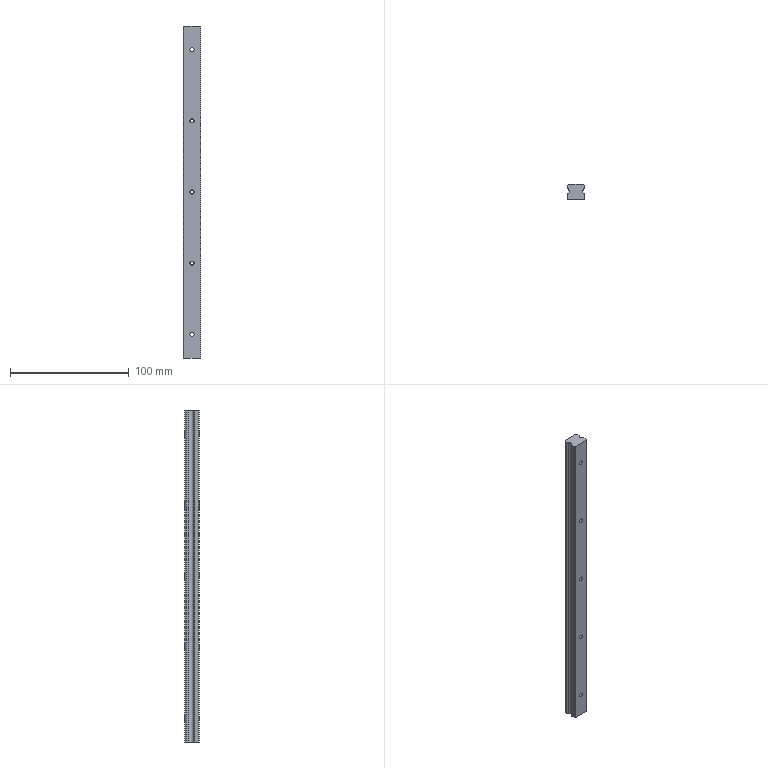Part | NX | features BREP 1 | 1 solid | 46 faces | box 15 x 12.5 x 280 mm | volume 46790 mm3 | cylinder 27 | plane 19 | commonest cylinder face diameters 3.5 x10 6 x10 3.4 x4 4 x3
STEP:
#1=CARTESIAN_POINT('',(0.,0.,-91.75));
#2=VERTEX_POINT('',#1);
#3=CARTESIAN_POINT('',(0.,0.,-88.25));
#4=VERTEX_POINT('',#3);
#5=CARTESIAN_POINT('',(0.,0.,-90.));
#6=DIRECTION('',(0.,1.,0.));
#7=DIRECTION('',(0.,0.,1.));
#8=AXIS2_PLACEMENT_3D('',#5,#6,#7);
#9=CIRCLE('',#8,1.75);
#10=EDGE_CURVE('',#2,#4,#9,.T.);
#11=ORIENTED_EDGE('',*,*,#10,.F.);
#12=CARTESIAN_POINT('',(0.,8.,-91.75));
#13=VERTEX_POINT('',#12);
#14=CARTESIAN_POINT('',(0.,0.,-91.75));
#15=DIRECTION('',(0.,1.,0.));
#16=VECTOR('',#15,1000.);
#17=LINE('',#14,#16);
#18=EDGE_CURVE('',#13,#2,#17,.F.);
#19=ORIENTED_EDGE('',*,*,#18,.F.);
#20=CARTESIAN_POINT('',(0.,8.,-88.25));
#21=VERTEX_POINT('',#20);
#22=CARTESIAN_POINT('',(0.,8.,-90.));
#23=DIRECTION('',(0.,1.,0.));
#24=DIRECTION('',(0.,0.,1.));
#25=AXIS2_PLACEMENT_3D('',#22,#23,#24);
#26=CIRCLE('',#25,1.75);
#27=EDGE_CURVE('',#13,#21,#26,.T.);
#28=ORIENTED_EDGE('',*,*,#27,.T.);
#29=CARTESIAN_POINT('',(0.,0.,-88.25));
#30=DIRECTION('',(0.,1.,0.));
#31=VECTOR('',#30,1000.);
#32=LINE('',#29,#31);
#33=EDGE_CURVE('',#21,#4,#32,.F.);
#34=ORIENTED_EDGE('',*,*,#33,.T.);
#35=EDGE_LOOP('',(#11,#19,#28,#34));
#36=FACE_BOUND('',#35,.T.);
#37=CARTESIAN_POINT('',(0.,0.,-90.));
#38=DIRECTION('',(0.,1.,0.));
#39=DIRECTION('',(0.,0.,1.));
#40=AXIS2_PLACEMENT_3D('',#37,#38,#39);
#41=CYLINDRICAL_SURFACE('',#40,1.75);
#42=ADVANCED_FACE('',(#36),#41,.F.);
#43=CARTESIAN_POINT('',(0.,8.,-93.));
#44=VERTEX_POINT('',#43);
#45=CARTESIAN_POINT('',(0.,8.,-87.));
#46=VERTEX_POINT('',#45);
#47=CARTESIAN_POINT('',(0.,8.,-90.));
#48=DIRECTION('',(0.,1.,0.));
#49=DIRECTION('',(0.,0.,1.));
#50=AXIS2_PLACEMENT_3D('',#47,#48,#49);
#51=CIRCLE('',#50,3.);
#52=EDGE_CURVE('',#44,#46,#51,.T.);
#53=ORIENTED_EDGE('',*,*,#52,.F.);
#54=CARTESIAN_POINT('',(0.,12.5,-93.));
#55=VERTEX_POINT('',#54);
#56=CARTESIAN_POINT('',(0.,0.,-93.));
#57=DIRECTION('',(0.,1.,0.));
#58=VECTOR('',#57,1000.);
#59=LINE('',#56,#58);
#60=EDGE_CURVE('',#55,#44,#59,.F.);
#61=ORIENTED_EDGE('',*,*,#60,.F.);
#62=CARTESIAN_POINT('',(0.,12.5,-87.));
#63=VERTEX_POINT('',#62);
#64=CARTESIAN_POINT('',(0.,12.5,-90.));
#65=DIRECTION('',(0.,1.,0.));
#66=DIRECTION('',(0.,0.,-1.));
#67=AXIS2_PLACEMENT_3D('',#64,#65,#66);
#68=CIRCLE('',#67,3.);
#69=EDGE_CURVE('',#55,#63,#68,.T.);
#70=ORIENTED_EDGE('',*,*,#69,.T.);
#71=CARTESIAN_POINT('',(0.,0.,-87.));
#72=DIRECTION('',(0.,1.,0.));
#73=VECTOR('',#72,1000.);
#74=LINE('',#71,#73);
#75=EDGE_CURVE('',#63,#46,#74,.F.);
#76=ORIENTED_EDGE('',*,*,#75,.T.);
#77=EDGE_LOOP('',(#53,#61,#70,#76));
#78=FACE_BOUND('',#77,.T.);
#79=CARTESIAN_POINT('',(0.,0.,-90.));
#80=DIRECTION('',(0.,1.,0.));
#81=DIRECTION('',(0.,0.,1.));
#82=AXIS2_PLACEMENT_3D('',#79,#80,#81);
#83=CYLINDRICAL_SURFACE('',#82,3.);
#84=ADVANCED_FACE('',(#78),#83,.F.);
#85=CARTESIAN_POINT('',(0.,0.,-31.75));
#86=VERTEX_POINT('',#85);
#87=CARTESIAN_POINT('',(0.,0.,-28.25));
#88=VERTEX_POINT('',#87);
#89=CARTESIAN_POINT('',(0.,0.,-30.));
#90=DIRECTION('',(0.,1.,0.));
#91=DIRECTION('',(0.,0.,1.));
#92=AXIS2_PLACEMENT_3D('',#89,#90,#91);
#93=CIRCLE('',#92,1.75);
#94=EDGE_CURVE('',#86,#88,#93,.T.);
#95=ORIENTED_EDGE('',*,*,#94,.F.);
#96=CARTESIAN_POINT('',(0.,8.,-31.75));
#97=VERTEX_POINT('',#96);
#98=CARTESIAN_POINT('',(0.,0.,-31.75));
#99=DIRECTION('',(0.,1.,0.));
#100=VECTOR('',#99,1000.);
#101=LINE('',#98,#100);
#102=EDGE_CURVE('',#97,#86,#101,.F.);
#103=ORIENTED_EDGE('',*,*,#102,.F.);
#104=CARTESIAN_POINT('',(0.,8.,-28.25));
#105=VERTEX_POINT('',#104);
#106=CARTESIAN_POINT('',(0.,8.,-30.));
#107=DIRECTION('',(0.,1.,0.));
#108=DIRECTION('',(0.,0.,1.));
#109=AXIS2_PLACEMENT_3D('',#106,#107,#108);
#110=CIRCLE('',#109,1.75);
#111=EDGE_CURVE('',#97,#105,#110,.T.);
#112=ORIENTED_EDGE('',*,*,#111,.T.);
#113=CARTESIAN_POINT('',(0.,0.,-28.25));
#114=DIRECTION('',(0.,1.,0.));
#115=VECTOR('',#114,1000.);
#116=LINE('',#113,#115);
#117=EDGE_CURVE('',#105,#88,#116,.F.);
#118=ORIENTED_EDGE('',*,*,#117,.T.);
#119=EDGE_LOOP('',(#95,#103,#112,#118));
#120=FACE_BOUND('',#119,.T.);
#121=CARTESIAN_POINT('',(0.,0.,-30.));
#122=DIRECTION('',(0.,1.,0.));
#123=DIRECTION('',(0.,0.,1.));
#124=AXIS2_PLACEMENT_3D('',#121,#122,#123);
#125=CYLINDRICAL_SURFACE('',#124,1.75);
#126=ADVANCED_FACE('',(#120),#125,.F.);
#127=CARTESIAN_POINT('',(0.,8.,-33.));
#128=VERTEX_POINT('',#127);
#129=CARTESIAN_POINT('',(0.,8.,-27.));
#130=VERTEX_POINT('',#129);
#131=CARTESIAN_POINT('',(0.,8.,-30.));
#132=DIRECTION('',(0.,1.,0.));
#133=DIRECTION('',(0.,0.,1.));
#134=AXIS2_PLACEMENT_3D('',#131,#132,#133);
#135=CIRCLE('',#134,3.);
#136=EDGE_CURVE('',#128,#130,#135,.T.);
#137=ORIENTED_EDGE('',*,*,#136,.F.);
#138=CARTESIAN_POINT('',(0.,12.5,-33.));
#139=VERTEX_POINT('',#138);
#140=CARTESIAN_POINT('',(0.,0.,-33.));
#141=DIRECTION('',(0.,1.,0.));
#142=VECTOR('',#141,1000.);
#143=LINE('',#140,#142);
#144=EDGE_CURVE('',#139,#128,#143,.F.);
#145=ORIENTED_EDGE('',*,*,#144,.F.);
#146=CARTESIAN_POINT('',(0.,12.5,-27.));
#147=VERTEX_POINT('',#146);
#148=CARTESIAN_POINT('',(0.,12.5,-30.));
#149=DIRECTION('',(0.,1.,0.));
#150=DIRECTION('',(0.,0.,-1.));
#151=AXIS2_PLACEMENT_3D('',#148,#149,#150);
#152=CIRCLE('',#151,3.);
#153=EDGE_CURVE('',#139,#147,#152,.T.);
#154=ORIENTED_EDGE('',*,*,#153,.T.);
#155=CARTESIAN_POINT('',(0.,0.,-27.));
#156=DIRECTION('',(0.,1.,0.));
#157=VECTOR('',#156,1000.);
#158=LINE('',#155,#157);
#159=EDGE_CURVE('',#147,#130,#158,.F.);
#160=ORIENTED_EDGE('',*,*,#159,.T.);
#161=EDGE_LOOP('',(#137,#145,#154,#160));
#162=FACE_BOUND('',#161,.T.);
#163=CARTESIAN_POINT('',(0.,0.,-30.));
#164=DIRECTION('',(0.,1.,0.));
#165=DIRECTION('',(0.,0.,1.));
#166=AXIS2_PLACEMENT_3D('',#163,#164,#165);
#167=CYLINDRICAL_SURFACE('',#166,3.);
#168=ADVANCED_FACE('',(#162),#167,.F.);
#169=CARTESIAN_POINT('',(0.,0.,28.25));
#170=VERTEX_POINT('',#169);
#171=CARTESIAN_POINT('',(0.,0.,31.75));
#172=VERTEX_POINT('',#171);
#173=CARTESIAN_POINT('',(0.,0.,30.));
#174=DIRECTION('',(0.,1.,0.));
#175=DIRECTION('',(0.,0.,1.));
#176=AXIS2_PLACEMENT_3D('',#173,#174,#175);
#177=CIRCLE('',#176,1.75);
#178=EDGE_CURVE('',#170,#172,#177,.T.);
#179=ORIENTED_EDGE('',*,*,#178,.F.);
#180=CARTESIAN_POINT('',(0.,8.,28.25));
#181=VERTEX_POINT('',#180);
#182=CARTESIAN_POINT('',(0.,0.,28.25));
#183=DIRECTION('',(0.,1.,0.));
#184=VECTOR('',#183,1000.);
#185=LINE('',#182,#184);
#186=EDGE_CURVE('',#181,#170,#185,.F.);
#187=ORIENTED_EDGE('',*,*,#186,.F.);
#188=CARTESIAN_POINT('',(0.,8.,31.75));
#189=VERTEX_POINT('',#188);
#190=CARTESIAN_POINT('',(0.,8.,30.));
#191=DIRECTION('',(0.,1.,0.));
#192=DIRECTION('',(0.,0.,1.));
#193=AXIS2_PLACEMENT_3D('',#190,#191,#192);
#194=CIRCLE('',#193,1.75);
#195=EDGE_CURVE('',#181,#189,#194,.T.);
#196=ORIENTED_EDGE('',*,*,#195,.T.);
#197=CARTESIAN_POINT('',(0.,0.,31.75));
#198=DIRECTION('',(0.,1.,0.));
#199=VECTOR('',#198,1000.);
#200=LINE('',#197,#199);
#201=EDGE_CURVE('',#189,#172,#200,.F.);
#202=ORIENTED_EDGE('',*,*,#201,.T.);
#203=EDGE_LOOP('',(#179,#187,#196,#202));
#204=FACE_BOUND('',#203,.T.);
#205=CARTESIAN_POINT('',(0.,0.,30.));
#206=DIRECTION('',(0.,1.,0.));
#207=DIRECTION('',(0.,0.,1.));
#208=AXIS2_PLACEMENT_3D('',#205,#206,#207);
#209=CYLINDRICAL_SURFACE('',#208,1.75);
#210=ADVANCED_FACE('',(#204),#209,.F.);
#211=CARTESIAN_POINT('',(0.,8.,27.));
#212=VERTEX_POINT('',#211);
#213=CARTESIAN_POINT('',(0.,8.,33.));
#214=VERTEX_POINT('',#213);
#215=CARTESIAN_POINT('',(0.,8.,30.));
#216=DIRECTION('',(0.,1.,0.));
#217=DIRECTION('',(0.,0.,1.));
#218=AXIS2_PLACEMENT_3D('',#215,#216,#217);
#219=CIRCLE('',#218,3.);
#220=EDGE_CURVE('',#212,#214,#219,.T.);
#221=ORIENTED_EDGE('',*,*,#220,.F.);
#222=CARTESIAN_POINT('',(0.,12.5,27.));
#223=VERTEX_POINT('',#222);
#224=CARTESIAN_POINT('',(0.,0.,27.));
#225=DIRECTION('',(0.,1.,0.));
#226=VECTOR('',#225,1000.);
#227=LINE('',#224,#226);
#228=EDGE_CURVE('',#223,#212,#227,.F.);
#229=ORIENTED_EDGE('',*,*,#228,.F.);
#230=CARTESIAN_POINT('',(0.,12.5,33.));
#231=VERTEX_POINT('',#230);
#232=CARTESIAN_POINT('',(0.,12.5,30.));
#233=DIRECTION('',(0.,1.,0.));
#234=DIRECTION('',(0.,0.,-1.));
#235=AXIS2_PLACEMENT_3D('',#232,#233,#234);
#236=CIRCLE('',#235,3.);
#237=EDGE_CURVE('',#223,#231,#236,.T.);
#238=ORIENTED_EDGE('',*,*,#237,.T.);
#239=CARTESIAN_POINT('',(0.,0.,33.));
#240=DIRECTION('',(0.,1.,0.));
#241=VECTOR('',#240,1000.);
#242=LINE('',#239,#241);
#243=EDGE_CURVE('',#231,#214,#242,.F.);
#244=ORIENTED_EDGE('',*,*,#243,.T.);
#245=EDGE_LOOP('',(#221,#229,#238,#244));
#246=FACE_BOUND('',#245,.T.);
#247=CARTESIAN_POINT('',(0.,0.,30.));
#248=DIRECTION('',(0.,1.,0.));
#249=DIRECTION('',(0.,0.,1.));
#250=AXIS2_PLACEMENT_3D('',#247,#248,#249);
#251=CYLINDRICAL_SURFACE('',#250,3.);
#252=ADVANCED_FACE('',(#246),#251,.F.);
#253=CARTESIAN_POINT('',(0.,0.,88.25));
#254=VERTEX_POINT('',#253);
#255=CARTESIAN_POINT('',(0.,0.,91.75));
#256=VERTEX_POINT('',#255);
#257=CARTESIAN_POINT('',(0.,0.,90.));
#258=DIRECTION('',(0.,1.,0.));
#259=DIRECTION('',(0.,0.,1.));
#260=AXIS2_PLACEMENT_3D('',#257,#258,#259);
#261=CIRCLE('',#260,1.75);
#262=EDGE_CURVE('',#254,#256,#261,.T.);
#263=ORIENTED_EDGE('',*,*,#262,.F.);
#264=CARTESIAN_POINT('',(0.,8.,88.25));
#265=VERTEX_POINT('',#264);
#266=CARTESIAN_POINT('',(0.,0.,88.25));
#267=DIRECTION('',(0.,1.,0.));
#268=VECTOR('',#267,1000.);
#269=LINE('',#266,#268);
#270=EDGE_CURVE('',#265,#254,#269,.F.);
#271=ORIENTED_EDGE('',*,*,#270,.F.);
#272=CARTESIAN_POINT('',(0.,8.,91.75));
#273=VERTEX_POINT('',#272);
#274=CARTESIAN_POINT('',(0.,8.,90.));
#275=DIRECTION('',(0.,1.,0.));
#276=DIRECTION('',(0.,0.,1.));
#277=AXIS2_PLACEMENT_3D('',#274,#275,#276);
#278=CIRCLE('',#277,1.75);
#279=EDGE_CURVE('',#265,#273,#278,.T.);
#280=ORIENTED_EDGE('',*,*,#279,.T.);
#281=CARTESIAN_POINT('',(0.,0.,91.75));
#282=DIRECTION('',(0.,1.,0.));
#283=VECTOR('',#282,1000.);
#284=LINE('',#281,#283);
#285=EDGE_CURVE('',#273,#256,#284,.F.);
#286=ORIENTED_EDGE('',*,*,#285,.T.);
#287=EDGE_LOOP('',(#263,#271,#280,#286));
#288=FACE_BOUND('',#287,.T.);
#289=CARTESIAN_POINT('',(0.,0.,90.));
#290=DIRECTION('',(0.,1.,0.));
#291=DIRECTION('',(0.,0.,1.));
#292=AXIS2_PLACEMENT_3D('',#289,#290,#291);
#293=CYLINDRICAL_SURFACE('',#292,1.75);
#294=ADVANCED_FACE('',(#288),#293,.F.);
#295=CARTESIAN_POINT('',(0.,8.,87.));
#296=VERTEX_POINT('',#295);
#297=CARTESIAN_POINT('',(0.,8.,93.));
#298=VERTEX_POINT('',#297);
#299=CARTESIAN_POINT('',(0.,8.,90.));
#300=DIRECTION('',(0.,1.,0.));
#301=DIRECTION('',(0.,0.,1.));
#302=AXIS2_PLACEMENT_3D('',#299,#300,#301);
#303=CIRCLE('',#302,3.);
#304=EDGE_CURVE('',#296,#298,#303,.T.);
#305=ORIENTED_EDGE('',*,*,#304,.F.);
#306=CARTESIAN_POINT('',(0.,12.5,87.));
#307=VERTEX_POINT('',#306);
#308=CARTESIAN_POINT('',(0.,0.,87.));
#309=DIRECTION('',(0.,1.,0.));
#310=VECTOR('',#309,1000.);
#311=LINE('',#308,#310);
#312=EDGE_CURVE('',#307,#296,#311,.F.);
#313=ORIENTED_EDGE('',*,*,#312,.F.);
#314=CARTESIAN_POINT('',(0.,12.5,93.));
#315=VERTEX_POINT('',#314);
#316=CARTESIAN_POINT('',(0.,12.5,90.));
#317=DIRECTION('',(0.,1.,0.));
#318=DIRECTION('',(0.,0.,-1.));
#319=AXIS2_PLACEMENT_3D('',#316,#317,#318);
#320=CIRCLE('',#319,3.);
#321=EDGE_CURVE('',#307,#315,#320,.T.);
#322=ORIENTED_EDGE('',*,*,#321,.T.);
#323=CARTESIAN_POINT('',(0.,0.,93.));
#324=DIRECTION('',(0.,1.,0.));
#325=VECTOR('',#324,1000.);
#326=LINE('',#323,#325);
#327=EDGE_CURVE('',#315,#298,#326,.F.);
#328=ORIENTED_EDGE('',*,*,#327,.T.);
#329=EDGE_LOOP('',(#305,#313,#322,#328));
#330=FACE_BOUND('',#329,.T.);
#331=CARTESIAN_POINT('',(0.,0.,90.));
#332=DIRECTION('',(0.,1.,0.));
#333=DIRECTION('',(0.,0.,1.));
#334=AXIS2_PLACEMENT_3D('',#331,#332,#333);
#335=CYLINDRICAL_SURFACE('',#334,3.);
#336=ADVANCED_FACE('',(#330),#335,.F.);
#337=CARTESIAN_POINT('',(0.,0.,-151.75));
#338=VERTEX_POINT('',#337);
#339=CARTESIAN_POINT('',(0.,0.,-148.25));
#340=VERTEX_POINT('',#339);
#341=CARTESIAN_POINT('',(0.,0.,-150.));
#342=DIRECTION('',(0.,1.,0.));
#343=DIRECTION('',(0.,0.,1.));
#344=AXIS2_PLACEMENT_3D('',#341,#342,#343);
#345=CIRCLE('',#344,1.75);
#346=EDGE_CURVE('',#338,#340,#345,.T.);
#347=ORIENTED_EDGE('',*,*,#346,.F.);
#348=CARTESIAN_POINT('',(0.,8.,-151.75));
#349=VERTEX_POINT('',#348);
#350=CARTESIAN_POINT('',(0.,0.,-151.75));
#351=DIRECTION('',(0.,1.,0.));
#352=VECTOR('',#351,1000.);
#353=LINE('',#350,#352);
#354=EDGE_CURVE('',#349,#338,#353,.F.);
#355=ORIENTED_EDGE('',*,*,#354,.F.);
#356=CARTESIAN_POINT('',(0.,8.,-148.25));
#357=VERTEX_POINT('',#356);
#358=CARTESIAN_POINT('',(0.,8.,-150.));
#359=DIRECTION('',(0.,1.,0.));
#360=DIRECTION('',(0.,0.,1.));
#361=AXIS2_PLACEMENT_3D('',#358,#359,#360);
#362=CIRCLE('',#361,1.75);
#363=EDGE_CURVE('',#349,#357,#362,.T.);
#364=ORIENTED_EDGE('',*,*,#363,.T.);
#365=CARTESIAN_POINT('',(0.,0.,-148.25));
#366=DIRECTION('',(0.,1.,0.));
#367=VECTOR('',#366,1000.);
#368=LINE('',#365,#367);
#369=EDGE_CURVE('',#357,#340,#368,.F.);
#370=ORIENTED_EDGE('',*,*,#369,.T.);
#371=EDGE_LOOP('',(#347,#355,#364,#370));
#372=FACE_BOUND('',#371,.T.);
#373=CARTESIAN_POINT('',(0.,0.,-150.));
#374=DIRECTION('',(0.,1.,0.));
#375=DIRECTION('',(0.,0.,1.));
#376=AXIS2_PLACEMENT_3D('',#373,#374,#375);
#377=CYLINDRICAL_SURFACE('',#376,1.75);
#378=ADVANCED_FACE('',(#372),#377,.F.);
#379=CARTESIAN_POINT('',(0.,8.,-153.));
#380=VERTEX_POINT('',#379);
#381=CARTESIAN_POINT('',(0.,8.,-147.));
#382=VERTEX_POINT('',#381);
#383=CARTESIAN_POINT('',(0.,8.,-150.));
#384=DIRECTION('',(0.,1.,0.));
#385=DIRECTION('',(0.,0.,1.));
#386=AXIS2_PLACEMENT_3D('',#383,#384,#385);
#387=CIRCLE('',#386,3.);
#388=EDGE_CURVE('',#380,#382,#387,.T.);
#389=ORIENTED_EDGE('',*,*,#388,.F.);
#390=CARTESIAN_POINT('',(0.,12.5,-153.));
#391=VERTEX_POINT('',#390);
#392=CARTESIAN_POINT('',(0.,0.,-153.));
#393=DIRECTION('',(0.,1.,0.));
#394=VECTOR('',#393,1000.);
#395=LINE('',#392,#394);
#396=EDGE_CURVE('',#391,#380,#395,.F.);
#397=ORIENTED_EDGE('',*,*,#396,.F.);
#398=CARTESIAN_POINT('',(0.,12.5,-147.));
#399=VERTEX_POINT('',#398);
#400=CARTESIAN_POINT('',(0.,12.5,-150.));
#401=DIRECTION('',(0.,1.,0.));
#402=DIRECTION('',(0.,0.,-1.));
#403=AXIS2_PLACEMENT_3D('',#400,#401,#402);
#404=CIRCLE('',#403,3.);
#405=EDGE_CURVE('',#391,#399,#404,.T.);
#406=ORIENTED_EDGE('',*,*,#405,.T.);
#407=CARTESIAN_POINT('',(0.,0.,-147.));
#408=DIRECTION('',(0.,1.,0.));
#409=VECTOR('',#408,1000.);
#410=LINE('',#407,#409);
#411=EDGE_CURVE('',#399,#382,#410,.F.);
#412=ORIENTED_EDGE('',*,*,#411,.T.);
#413=EDGE_LOOP('',(#389,#397,#406,#412));
#414=FACE_BOUND('',#413,.T.);
#415=CARTESIAN_POINT('',(0.,0.,-150.));
#416=DIRECTION('',(0.,1.,0.));
#417=DIRECTION('',(0.,0.,1.));
#418=AXIS2_PLACEMENT_3D('',#415,#416,#417);
#419=CYLINDRICAL_SURFACE('',#418,3.);
#420=ADVANCED_FACE('',(#414),#419,.F.);
#421=CARTESIAN_POINT('',(6.256,8.066,110.));
#422=VERTEX_POINT('',#421);
#423=CARTESIAN_POINT('',(5.5,6.5,110.));
#424=VERTEX_POINT('',#423);
#425=CARTESIAN_POINT('',(7.5,6.5,110.));
#426=DIRECTION('',(0.,0.,1.));
#427=DIRECTION('',(-1.,0.,0.));
#428=AXIS2_PLACEMENT_3D('',#425,#426,#427);
#429=CIRCLE('',#428,2.);
#430=EDGE_CURVE('',#422,#424,#429,.T.);
#431=ORIENTED_EDGE('',*,*,#430,.T.);
#432=CARTESIAN_POINT('',(5.5,6.5,-170.));
#433=VERTEX_POINT('',#432);
#434=CARTESIAN_POINT('',(5.5,6.5,170.));
#435=DIRECTION('',(0.,0.,-1.));
#436=VECTOR('',#435,1000.);
#437=LINE('',#434,#436);
#438=EDGE_CURVE('',#424,#433,#437,.T.);
#439=ORIENTED_EDGE('',*,*,#438,.T.);
#440=CARTESIAN_POINT('',(6.256,8.066,-170.));
#441=VERTEX_POINT('',#440);
#442=CARTESIAN_POINT('',(7.5,6.5,-170.));
#443=DIRECTION('',(0.,0.,-1.));
#444=DIRECTION('',(-1.,0.,0.));
#445=AXIS2_PLACEMENT_3D('',#442,#443,#444);
#446=CIRCLE('',#445,2.);
#447=EDGE_CURVE('',#433,#441,#446,.T.);
#448=ORIENTED_EDGE('',*,*,#447,.T.);
#449=CARTESIAN_POINT('',(6.256,8.066,170.));
#450=DIRECTION('',(0.,0.,-1.));
#451=VECTOR('',#450,1000.);
#452=LINE('',#449,#451);
#453=EDGE_CURVE('',#422,#441,#452,.T.);
#454=ORIENTED_EDGE('',*,*,#453,.F.);
#455=EDGE_LOOP('',(#431,#439,#448,#454));
#456=FACE_BOUND('',#455,.T.);
#457=CARTESIAN_POINT('',(7.5,6.5,170.));
#458=DIRECTION('',(0.,0.,-1.));
#459=DIRECTION('',(-1.,0.,0.));
#460=AXIS2_PLACEMENT_3D('',#457,#458,#459);
#461=CYLINDRICAL_SURFACE('',#460,2.);
#462=ADVANCED_FACE('',(#456),#461,.F.);
#463=CARTESIAN_POINT('',(7.,0.,110.));
#464=VERTEX_POINT('',#463);
#465=CARTESIAN_POINT('',(7.,0.,-170.));
#466=VERTEX_POINT('',#465);
#467=CARTESIAN_POINT('',(7.,0.,170.));
#468=DIRECTION('',(0.,0.,-1.));
#469=VECTOR('',#468,1000.);
#470=LINE('',#467,#469);
#471=EDGE_CURVE('',#464,#466,#470,.T.);
#472=ORIENTED_EDGE('',*,*,#471,.F.);
#473=CARTESIAN_POINT('',(-7.,0.,110.));
#474=VERTEX_POINT('',#473);
#475=CARTESIAN_POINT('',(7.5,0.,110.));
#476=DIRECTION('',(-1.,0.,0.));
#477=VECTOR('',#476,1000.);
#478=LINE('',#475,#477);
#479=EDGE_CURVE('',#464,#474,#478,.T.);
#480=ORIENTED_EDGE('',*,*,#479,.T.);
#481=CARTESIAN_POINT('',(-7.,0.,-170.));
#482=VERTEX_POINT('',#481);
#483=CARTESIAN_POINT('',(-7.,0.,170.));
#484=DIRECTION('',(0.,0.,-1.));
#485=VECTOR('',#484,1000.);
#486=LINE('',#483,#485);
#487=EDGE_CURVE('',#474,#482,#486,.T.);
#488=ORIENTED_EDGE('',*,*,#487,.T.);
#489=CARTESIAN_POINT('',(-7.,0.,-170.));
#490=DIRECTION('',(1.,0.,0.));
#491=VECTOR('',#490,1000.);
#492=LINE('',#489,#491);
#493=EDGE_CURVE('',#482,#466,#492,.T.);
#494=ORIENTED_EDGE('',*,*,#493,.T.);
#495=EDGE_LOOP('',(#472,#480,#488,#494));
#496=FACE_BOUND('',#495,.T.);
#497=CARTESIAN_POINT('',(0.,0.,-30.));
#498=DIRECTION('',(0.,1.,0.));
#499=DIRECTION('',(0.,0.,1.));
#500=AXIS2_PLACEMENT_3D('',#497,#498,#499);
#501=CIRCLE('',#500,1.75);
#502=EDGE_CURVE('',#88,#86,#501,.T.);
#503=ORIENTED_EDGE('',*,*,#502,.T.);
#504=ORIENTED_EDGE('',*,*,#94,.T.);
#505=EDGE_LOOP('',(#503,#504));
#506=FACE_BOUND('',#505,.T.);
#507=CARTESIAN_POINT('',(0.,0.,90.));
#508=DIRECTION('',(0.,1.,0.));
#509=DIRECTION('',(0.,0.,1.));
#510=AXIS2_PLACEMENT_3D('',#507,#508,#509);
#511=CIRCLE('',#510,1.75);
#512=EDGE_CURVE('',#256,#254,#511,.T.);
#513=ORIENTED_EDGE('',*,*,#512,.T.);
#514=ORIENTED_EDGE('',*,*,#262,.T.);
#515=EDGE_LOOP('',(#513,#514));
#516=FACE_BOUND('',#515,.T.);
#517=CARTESIAN_POINT('',(0.,0.,-150.));
#518=DIRECTION('',(0.,1.,0.));
#519=DIRECTION('',(0.,0.,1.));
#520=AXIS2_PLACEMENT_3D('',#517,#518,#519);
#521=CIRCLE('',#520,1.75);
#522=EDGE_CURVE('',#340,#338,#521,.T.);
#523=ORIENTED_EDGE('',*,*,#522,.T.);
#524=ORIENTED_EDGE('',*,*,#346,.T.);
#525=EDGE_LOOP('',(#523,#524));
#526=FACE_BOUND('',#525,.T.);
#527=CARTESIAN_POINT('',(0.,0.,30.));
#528=DIRECTION('',(0.,1.,0.));
#529=DIRECTION('',(0.,0.,1.));
#530=AXIS2_PLACEMENT_3D('',#527,#528,#529);
#531=CIRCLE('',#530,1.75);
#532=EDGE_CURVE('',#172,#170,#531,.T.);
#533=ORIENTED_EDGE('',*,*,#532,.T.);
#534=ORIENTED_EDGE('',*,*,#178,.T.);
#535=EDGE_LOOP('',(#533,#534));
#536=FACE_BOUND('',#535,.T.);
#537=CARTESIAN_POINT('',(0.,0.,-90.));
#538=DIRECTION('',(0.,1.,0.));
#539=DIRECTION('',(0.,0.,1.));
#540=AXIS2_PLACEMENT_3D('',#537,#538,#539);
#541=CIRCLE('',#540,1.75);
#542=EDGE_CURVE('',#4,#2,#541,.T.);
#543=ORIENTED_EDGE('',*,*,#542,.T.);
#544=ORIENTED_EDGE('',*,*,#10,.T.);
#545=EDGE_LOOP('',(#543,#544));
#546=FACE_BOUND('',#545,.T.);
#547=CARTESIAN_POINT('',(-7.,0.,170.));
#548=DIRECTION('',(0.,1.,0.));
#549=DIRECTION('',(1.,0.,0.));
#550=AXIS2_PLACEMENT_3D('',#547,#548,#549);
#551=PLANE('',#550);
#552=ADVANCED_FACE('',(#496,#506,#516,#526,#536,#546),#551,.F.);
#553=CARTESIAN_POINT('',(-6.1,12.5,110.));
#554=VERTEX_POINT('',#553);
#555=CARTESIAN_POINT('',(-6.1,12.5,-170.));
#556=VERTEX_POINT('',#555);
#557=CARTESIAN_POINT('',(-6.1,12.5,170.));
#558=DIRECTION('',(0.,0.,-1.));
#559=VECTOR('',#558,1000.);
#560=LINE('',#557,#559);
#561=EDGE_CURVE('',#554,#556,#560,.T.);
#562=ORIENTED_EDGE('',*,*,#561,.F.);
#563=CARTESIAN_POINT('',(6.1,12.5,110.));
#564=VERTEX_POINT('',#563);
#565=CARTESIAN_POINT('',(7.5,12.5,110.));
#566=DIRECTION('',(-1.,0.,0.));
#567=VECTOR('',#566,1000.);
#568=LINE('',#565,#567);
#569=EDGE_CURVE('',#564,#554,#568,.T.);
#570=ORIENTED_EDGE('',*,*,#569,.F.);
#571=CARTESIAN_POINT('',(6.1,12.5,-170.));
#572=VERTEX_POINT('',#571);
#573=CARTESIAN_POINT('',(6.1,12.5,170.));
#574=DIRECTION('',(0.,0.,-1.));
#575=VECTOR('',#574,1000.);
#576=LINE('',#573,#575);
#577=EDGE_CURVE('',#564,#572,#576,.T.);
#578=ORIENTED_EDGE('',*,*,#577,.T.);
#579=CARTESIAN_POINT('',(6.1,12.5,-170.));
#580=DIRECTION('',(-1.,0.,0.));
#581=VECTOR('',#580,1000.);
#582=LINE('',#579,#581);
#583=EDGE_CURVE('',#572,#556,#582,.T.);
#584=ORIENTED_EDGE('',*,*,#583,.T.);
#585=EDGE_LOOP('',(#562,#570,#578,#584));
#586=FACE_BOUND('',#585,.T.);
#587=CARTESIAN_POINT('',(0.,12.5,-30.));
#588=DIRECTION('',(0.,1.,0.));
#589=DIRECTION('',(0.,0.,-1.));
#590=AXIS2_PLACEMENT_3D('',#587,#588,#589);
#591=CIRCLE('',#590,3.);
#592=EDGE_CURVE('',#147,#139,#591,.T.);
#593=ORIENTED_EDGE('',*,*,#592,.F.);
#594=ORIENTED_EDGE('',*,*,#153,.F.);
#595=EDGE_LOOP('',(#593,#594));
#596=FACE_BOUND('',#595,.T.);
#597=CARTESIAN_POINT('',(0.,12.5,90.));
#598=DIRECTION('',(0.,1.,0.));
#599=DIRECTION('',(0.,0.,-1.));
#600=AXIS2_PLACEMENT_3D('',#597,#598,#599);
#601=CIRCLE('',#600,3.);
#602=EDGE_CURVE('',#315,#307,#601,.T.);
#603=ORIENTED_EDGE('',*,*,#602,.F.);
#604=ORIENTED_EDGE('',*,*,#321,.F.);
#605=EDGE_LOOP('',(#603,#604));
#606=FACE_BOUND('',#605,.T.);
#607=CARTESIAN_POINT('',(0.,12.5,-150.));
#608=DIRECTION('',(0.,1.,0.));
#609=DIRECTION('',(0.,0.,-1.));
#610=AXIS2_PLACEMENT_3D('',#607,#608,#609);
#611=CIRCLE('',#610,3.);
#612=EDGE_CURVE('',#399,#391,#611,.T.);
#613=ORIENTED_EDGE('',*,*,#612,.F.);
#614=ORIENTED_EDGE('',*,*,#405,.F.);
#615=EDGE_LOOP('',(#613,#614));
#616=FACE_BOUND('',#615,.T.);
#617=CARTESIAN_POINT('',(0.,12.5,30.));
#618=DIRECTION('',(0.,1.,0.));
#619=DIRECTION('',(0.,0.,-1.));
#620=AXIS2_PLACEMENT_3D('',#617,#618,#619);
#621=CIRCLE('',#620,3.);
#622=EDGE_CURVE('',#231,#223,#621,.T.);
#623=ORIENTED_EDGE('',*,*,#622,.F.);
#624=ORIENTED_EDGE('',*,*,#237,.F.);
#625=EDGE_LOOP('',(#623,#624));
#626=FACE_BOUND('',#625,.T.);
#627=CARTESIAN_POINT('',(0.,12.5,-90.));
#628=DIRECTION('',(0.,1.,0.));
#629=DIRECTION('',(0.,0.,-1.));
#630=AXIS2_PLACEMENT_3D('',#627,#628,#629);
#631=CIRCLE('',#630,3.);
#632=EDGE_CURVE('',#63,#55,#631,.T.);
#633=ORIENTED_EDGE('',*,*,#632,.F.);
#634=ORIENTED_EDGE('',*,*,#69,.F.);
#635=EDGE_LOOP('',(#633,#634));
#636=FACE_BOUND('',#635,.T.);
#637=CARTESIAN_POINT('',(6.1,12.5,170.));
#638=DIRECTION('',(0.,-1.,0.));
#639=DIRECTION('',(0.,0.,-1.));
#640=AXIS2_PLACEMENT_3D('',#637,#638,#639);
#641=PLANE('',#640);
#642=ADVANCED_FACE('',(#586,#596,#606,#616,#626,#636),#641,.F.);
#643=CARTESIAN_POINT('',(-7.5,4.,110.));
#644=VERTEX_POINT('',#643);
#645=CARTESIAN_POINT('',(-7.5,4.,-170.));
#646=VERTEX_POINT('',#645);
#647=CARTESIAN_POINT('',(-7.5,4.,170.));
#648=DIRECTION('',(0.,0.,-1.));
#649=VECTOR('',#648,1000.);
#650=LINE('',#647,#649);
#651=EDGE_CURVE('',#644,#646,#650,.T.);
#652=ORIENTED_EDGE('',*,*,#651,.F.);
#653=CARTESIAN_POINT('',(-6.911,4.589,110.));
#654=VERTEX_POINT('',#653);
#655=CARTESIAN_POINT('',(-6.911,4.589,110.));
#656=DIRECTION('',(0.7071,0.7071,0.));
#657=VECTOR('',#656,1000.);
#658=LINE('',#655,#657);
#659=EDGE_CURVE('',#644,#654,#658,.T.);
#660=ORIENTED_EDGE('',*,*,#659,.T.);
#661=CARTESIAN_POINT('',(-6.911,4.589,-170.));
#662=VERTEX_POINT('',#661);
#663=CARTESIAN_POINT('',(-6.911,4.589,170.));
#664=DIRECTION('',(0.,0.,-1.));
#665=VECTOR('',#664,1000.);
#666=LINE('',#663,#665);
#667=EDGE_CURVE('',#654,#662,#666,.T.);
#668=ORIENTED_EDGE('',*,*,#667,.T.);
#669=CARTESIAN_POINT('',(-6.911,4.589,-170.));
#670=DIRECTION('',(-0.7071,-0.7071,0.));
#671=VECTOR('',#670,1000.);
#672=LINE('',#669,#671);
#673=EDGE_CURVE('',#662,#646,#672,.T.);
#674=ORIENTED_EDGE('',*,*,#673,.T.);
#675=EDGE_LOOP('',(#652,#660,#668,#674));
#676=FACE_BOUND('',#675,.T.);
#677=CARTESIAN_POINT('',(-6.911,4.589,170.));
#678=DIRECTION('',(0.7071,-0.7071,0.));
#679=DIRECTION('',(0.,0.,-1.));
#680=AXIS2_PLACEMENT_3D('',#677,#678,#679);
#681=PLANE('',#680);
#682=ADVANCED_FACE('',(#676),#681,.F.);
#683=CARTESIAN_POINT('',(-7.5,0.5,110.));
#684=VERTEX_POINT('',#683);
#685=CARTESIAN_POINT('',(-7.5,0.5,-170.));
#686=VERTEX_POINT('',#685);
#687=CARTESIAN_POINT('',(-7.5,0.5,170.));
#688=DIRECTION('',(0.,0.,-1.));
#689=VECTOR('',#688,1000.);
#690=LINE('',#687,#689);
#691=EDGE_CURVE('',#684,#686,#690,.T.);
#692=ORIENTED_EDGE('',*,*,#691,.F.);
#693=CARTESIAN_POINT('',(-7.5,0.,110.));
#694=DIRECTION('',(0.,1.,0.));
#695=VECTOR('',#694,1000.);
#696=LINE('',#693,#695);
#697=EDGE_CURVE('',#684,#644,#696,.T.);
#698=ORIENTED_EDGE('',*,*,#697,.T.);
#699=ORIENTED_EDGE('',*,*,#651,.T.);
#700=CARTESIAN_POINT('',(-7.5,4.,-170.));
#701=DIRECTION('',(0.,-1.,0.));
#702=VECTOR('',#701,1000.);
#703=LINE('',#700,#702);
#704=EDGE_CURVE('',#646,#686,#703,.T.);
#705=ORIENTED_EDGE('',*,*,#704,.T.);
#706=EDGE_LOOP('',(#692,#698,#699,#705));
#707=FACE_BOUND('',#706,.T.);
#708=CARTESIAN_POINT('',(-7.5,4.,170.));
#709=DIRECTION('',(1.,0.,0.));
#710=DIRECTION('',(0.,1.,0.));
#711=AXIS2_PLACEMENT_3D('',#708,#709,#710);
#712=PLANE('',#711);
#713=ADVANCED_FACE('',(#707),#712,.F.);
#714=ORIENTED_EDGE('',*,*,#487,.F.);
#715=CARTESIAN_POINT('',(-7.5,0.5,110.));
#716=DIRECTION('',(-0.7071,0.7071,0.));
#717=VECTOR('',#716,1000.);
#718=LINE('',#715,#717);
#719=EDGE_CURVE('',#474,#684,#718,.T.);
#720=ORIENTED_EDGE('',*,*,#719,.T.);
#721=ORIENTED_EDGE('',*,*,#691,.T.);
#722=CARTESIAN_POINT('',(-7.5,0.5,-170.));
#723=DIRECTION('',(0.7071,-0.7071,0.));
#724=VECTOR('',#723,1000.);
#725=LINE('',#722,#724);
#726=EDGE_CURVE('',#686,#482,#725,.T.);
#727=ORIENTED_EDGE('',*,*,#726,.T.);
#728=EDGE_LOOP('',(#714,#720,#721,#727));
#729=FACE_BOUND('',#728,.T.);
#730=CARTESIAN_POINT('',(-7.5,0.5,170.));
#731=DIRECTION('',(0.7071,0.7071,0.));
#732=DIRECTION('',(0.,0.,-1.));
#733=AXIS2_PLACEMENT_3D('',#730,#731,#732);
#734=PLANE('',#733);
#735=ADVANCED_FACE('',(#729),#734,.F.);
#736=CARTESIAN_POINT('',(7.5,0.5,110.));
#737=VERTEX_POINT('',#736);
#738=CARTESIAN_POINT('',(7.5,0.5,-170.));
#739=VERTEX_POINT('',#738);
#740=CARTESIAN_POINT('',(7.5,0.5,170.));
#741=DIRECTION('',(0.,0.,-1.));
#742=VECTOR('',#741,1000.);
#743=LINE('',#740,#742);
#744=EDGE_CURVE('',#737,#739,#743,.T.);
#745=ORIENTED_EDGE('',*,*,#744,.F.);
#746=CARTESIAN_POINT('',(7.,0.,110.));
#747=DIRECTION('',(-0.7071,-0.7071,0.));
#748=VECTOR('',#747,1000.);
#749=LINE('',#746,#748);
#750=EDGE_CURVE('',#737,#464,#749,.T.);
#751=ORIENTED_EDGE('',*,*,#750,.T.);
#752=ORIENTED_EDGE('',*,*,#471,.T.);
#753=CARTESIAN_POINT('',(7.,0.,-170.));
#754=DIRECTION('',(0.7071,0.7071,0.));
#755=VECTOR('',#754,1000.);
#756=LINE('',#753,#755);
#757=EDGE_CURVE('',#466,#739,#756,.T.);
#758=ORIENTED_EDGE('',*,*,#757,.T.);
#759=EDGE_LOOP('',(#745,#751,#752,#758));
#760=FACE_BOUND('',#759,.T.);
#761=CARTESIAN_POINT('',(7.,0.,170.));
#762=DIRECTION('',(-0.7071,0.7071,0.));
#763=DIRECTION('',(0.,0.,1.));
#764=AXIS2_PLACEMENT_3D('',#761,#762,#763);
#765=PLANE('',#764);
#766=ADVANCED_FACE('',(#760),#765,.F.);
#767=CARTESIAN_POINT('',(7.5,4.,110.));
#768=VERTEX_POINT('',#767);
#769=CARTESIAN_POINT('',(7.5,4.,-170.));
#770=VERTEX_POINT('',#769);
#771=CARTESIAN_POINT('',(7.5,4.,170.));
#772=DIRECTION('',(0.,0.,-1.));
#773=VECTOR('',#772,1000.);
#774=LINE('',#771,#773);
#775=EDGE_CURVE('',#768,#770,#774,.T.);
#776=ORIENTED_EDGE('',*,*,#775,.F.);
#777=CARTESIAN_POINT('',(7.5,0.,110.));
#778=DIRECTION('',(0.,1.,0.));
#779=VECTOR('',#778,1000.);
#780=LINE('',#777,#779);
#781=EDGE_CURVE('',#737,#768,#780,.T.);
#782=ORIENTED_EDGE('',*,*,#781,.F.);
#783=ORIENTED_EDGE('',*,*,#744,.T.);
#784=CARTESIAN_POINT('',(7.5,0.5,-170.));
#785=DIRECTION('',(0.,1.,0.));
#786=VECTOR('',#785,1000.);
#787=LINE('',#784,#786);
#788=EDGE_CURVE('',#739,#770,#787,.T.);
#789=ORIENTED_EDGE('',*,*,#788,.T.);
#790=EDGE_LOOP('',(#776,#782,#783,#789));
#791=FACE_BOUND('',#790,.T.);
#792=CARTESIAN_POINT('',(7.5,0.5,170.));
#793=DIRECTION('',(-1.,0.,0.));
#794=DIRECTION('',(0.,0.,1.));
#795=AXIS2_PLACEMENT_3D('',#792,#793,#794);
#796=PLANE('',#795);
#797=ADVANCED_FACE('',(#791),#796,.F.);
#798=CARTESIAN_POINT('',(6.911,4.589,110.));
#799=VERTEX_POINT('',#798);
#800=CARTESIAN_POINT('',(6.911,4.589,-170.));
#801=VERTEX_POINT('',#800);
#802=CARTESIAN_POINT('',(6.911,4.589,170.));
#803=DIRECTION('',(0.,0.,-1.));
#804=VECTOR('',#803,1000.);
#805=LINE('',#802,#804);
#806=EDGE_CURVE('',#799,#801,#805,.T.);
#807=ORIENTED_EDGE('',*,*,#806,.F.);
#808=CARTESIAN_POINT('',(7.5,4.,110.));
#809=DIRECTION('',(0.7071,-0.7071,0.));
#810=VECTOR('',#809,1000.);
#811=LINE('',#808,#810);
#812=EDGE_CURVE('',#799,#768,#811,.T.);
#813=ORIENTED_EDGE('',*,*,#812,.T.);
#814=ORIENTED_EDGE('',*,*,#775,.T.);
#815=CARTESIAN_POINT('',(7.5,4.,-170.));
#816=DIRECTION('',(-0.7071,0.7071,0.));
#817=VECTOR('',#816,1000.);
#818=LINE('',#815,#817);
#819=EDGE_CURVE('',#770,#801,#818,.T.);
#820=ORIENTED_EDGE('',*,*,#819,.T.);
#821=EDGE_LOOP('',(#807,#813,#814,#820));
#822=FACE_BOUND('',#821,.T.);
#823=CARTESIAN_POINT('',(7.5,4.,170.));
#824=DIRECTION('',(-0.7071,-0.7071,0.));
#825=DIRECTION('',(-0.7071,0.7071,0.));
#826=AXIS2_PLACEMENT_3D('',#823,#824,#825);
#827=PLANE('',#826);
#828=ADVANCED_FACE('',(#822),#827,.F.);
#829=ORIENTED_EDGE('',*,*,#438,.F.);
#830=CARTESIAN_POINT('',(7.5,6.5,110.));
#831=DIRECTION('',(0.,0.,1.));
#832=DIRECTION('',(-1.,0.,0.));
#833=AXIS2_PLACEMENT_3D('',#830,#831,#832);
#834=CIRCLE('',#833,2.);
#835=EDGE_CURVE('',#424,#799,#834,.T.);
#836=ORIENTED_EDGE('',*,*,#835,.T.);
#837=ORIENTED_EDGE('',*,*,#806,.T.);
#838=CARTESIAN_POINT('',(7.5,6.5,-170.));
#839=DIRECTION('',(0.,0.,-1.));
#840=DIRECTION('',(-1.,0.,0.));
#841=AXIS2_PLACEMENT_3D('',#838,#839,#840);
#842=CIRCLE('',#841,2.);
#843=EDGE_CURVE('',#801,#433,#842,.T.);
#844=ORIENTED_EDGE('',*,*,#843,.T.);
#845=EDGE_LOOP('',(#829,#836,#837,#844));
#846=FACE_BOUND('',#845,.T.);
#847=CARTESIAN_POINT('',(7.5,6.5,170.));
#848=DIRECTION('',(0.,0.,-1.));
#849=DIRECTION('',(-1.,0.,0.));
#850=AXIS2_PLACEMENT_3D('',#847,#848,#849);
#851=CYLINDRICAL_SURFACE('',#850,2.);
#852=ADVANCED_FACE('',(#846),#851,.F.);
#853=CARTESIAN_POINT('',(7.5,9.416,110.));
#854=VERTEX_POINT('',#853);
#855=CARTESIAN_POINT('',(7.5,9.416,-170.));
#856=VERTEX_POINT('',#855);
#857=CARTESIAN_POINT('',(7.5,9.416,170.));
#858=DIRECTION('',(0.,0.,-1.));
#859=VECTOR('',#858,1000.);
#860=LINE('',#857,#859);
#861=EDGE_CURVE('',#854,#856,#860,.T.);
#862=ORIENTED_EDGE('',*,*,#861,.F.);
#863=CARTESIAN_POINT('',(7.93,7.771,110.));
#864=DIRECTION('',(0.,0.,1.));
#865=DIRECTION('',(-1.,0.,0.));
#866=AXIS2_PLACEMENT_3D('',#863,#864,#865);
#867=CIRCLE('',#866,1.7);
#868=EDGE_CURVE('',#854,#422,#867,.T.);
#869=ORIENTED_EDGE('',*,*,#868,.T.);
#870=ORIENTED_EDGE('',*,*,#453,.T.);
#871=CARTESIAN_POINT('',(7.93,7.771,-170.));
#872=DIRECTION('',(0.,0.,-1.));
#873=DIRECTION('',(-1.,0.,0.));
#874=AXIS2_PLACEMENT_3D('',#871,#872,#873);
#875=CIRCLE('',#874,1.7);
#876=EDGE_CURVE('',#441,#856,#875,.T.);
#877=ORIENTED_EDGE('',*,*,#876,.T.);
#878=EDGE_LOOP('',(#862,#869,#870,#877));
#879=FACE_BOUND('',#878,.T.);
#880=CARTESIAN_POINT('',(7.93,7.771,170.));
#881=DIRECTION('',(0.,0.,-1.));
#882=DIRECTION('',(-1.,0.,0.));
#883=AXIS2_PLACEMENT_3D('',#880,#881,#882);
#884=CYLINDRICAL_SURFACE('',#883,1.7);
#885=ADVANCED_FACE('',(#879),#884,.F.);
#886=CARTESIAN_POINT('',(7.5,11.285,110.));
#887=VERTEX_POINT('',#886);
#888=CARTESIAN_POINT('',(7.5,11.285,-170.));
#889=VERTEX_POINT('',#888);
#890=CARTESIAN_POINT('',(7.5,11.285,170.));
#891=DIRECTION('',(0.,0.,-1.));
#892=VECTOR('',#891,1000.);
#893=LINE('',#890,#892);
#894=EDGE_CURVE('',#887,#889,#893,.T.);
#895=ORIENTED_EDGE('',*,*,#894,.F.);
#896=CARTESIAN_POINT('',(7.5,0.,110.));
#897=DIRECTION('',(0.,1.,0.));
#898=VECTOR('',#897,1000.);
#899=LINE('',#896,#898);
#900=EDGE_CURVE('',#854,#887,#899,.T.);
#901=ORIENTED_EDGE('',*,*,#900,.F.);
#902=ORIENTED_EDGE('',*,*,#861,.T.);
#903=CARTESIAN_POINT('',(7.5,9.416,-170.));
#904=DIRECTION('',(0.,1.,0.));
#905=VECTOR('',#904,1000.);
#906=LINE('',#903,#905);
#907=EDGE_CURVE('',#856,#889,#906,.T.);
#908=ORIENTED_EDGE('',*,*,#907,.T.);
#909=EDGE_LOOP('',(#895,#901,#902,#908));
#910=FACE_BOUND('',#909,.T.);
#911=CARTESIAN_POINT('',(7.5,9.416,170.));
#912=DIRECTION('',(-1.,0.,0.));
#913=DIRECTION('',(0.,0.,1.));
#914=AXIS2_PLACEMENT_3D('',#911,#912,#913);
#915=PLANE('',#914);
#916=ADVANCED_FACE('',(#910),#915,.F.);
#917=CARTESIAN_POINT('',(6.325,12.37,110.));
#918=VERTEX_POINT('',#917);
#919=CARTESIAN_POINT('',(6.325,12.37,-170.));
#920=VERTEX_POINT('',#919);
#921=CARTESIAN_POINT('',(6.325,12.37,170.));
#922=DIRECTION('',(0.,0.,-1.));
#923=VECTOR('',#922,1000.);
#924=LINE('',#921,#923);
#925=EDGE_CURVE('',#918,#920,#924,.T.);
#926=ORIENTED_EDGE('',*,*,#925,.F.);
#927=CARTESIAN_POINT('',(7.93,12.93,110.));
#928=DIRECTION('',(0.,0.,1.));
#929=DIRECTION('',(-1.,0.,0.));
#930=AXIS2_PLACEMENT_3D('',#927,#928,#929);
#931=CIRCLE('',#930,1.7);
#932=EDGE_CURVE('',#918,#887,#931,.T.);
#933=ORIENTED_EDGE('',*,*,#932,.T.);
#934=ORIENTED_EDGE('',*,*,#894,.T.);
#935=CARTESIAN_POINT('',(7.93,12.93,-170.));
#936=DIRECTION('',(0.,0.,-1.));
#937=DIRECTION('',(-1.,0.,0.));
#938=AXIS2_PLACEMENT_3D('',#935,#936,#937);
#939=CIRCLE('',#938,1.7);
#940=EDGE_CURVE('',#889,#920,#939,.T.);
#941=ORIENTED_EDGE('',*,*,#940,.T.);
#942=EDGE_LOOP('',(#926,#933,#934,#941));
#943=FACE_BOUND('',#942,.T.);
#944=CARTESIAN_POINT('',(7.93,12.93,170.));
#945=DIRECTION('',(0.,0.,-1.));
#946=DIRECTION('',(-1.,0.,0.));
#947=AXIS2_PLACEMENT_3D('',#944,#945,#946);
#948=CYLINDRICAL_SURFACE('',#947,1.7);
#949=ADVANCED_FACE('',(#943),#948,.F.);
#950=ORIENTED_EDGE('',*,*,#577,.F.);
#951=CARTESIAN_POINT('',(6.325,12.37,110.));
#952=DIRECTION('',(0.866,-0.5,0.));
#953=VECTOR('',#952,1000.);
#954=LINE('',#951,#953);
#955=EDGE_CURVE('',#564,#918,#954,.T.);
#956=ORIENTED_EDGE('',*,*,#955,.T.);
#957=ORIENTED_EDGE('',*,*,#925,.T.);
#958=CARTESIAN_POINT('',(6.325,12.37,-170.));
#959=DIRECTION('',(-0.866,0.5,0.));
#960=VECTOR('',#959,1000.);
#961=LINE('',#958,#960);
#962=EDGE_CURVE('',#920,#572,#961,.T.);
#963=ORIENTED_EDGE('',*,*,#962,.T.);
#964=EDGE_LOOP('',(#950,#956,#957,#963));
#965=FACE_BOUND('',#964,.T.);
#966=CARTESIAN_POINT('',(6.325,12.37,170.));
#967=DIRECTION('',(-0.5,-0.866,0.));
#968=DIRECTION('',(-0.866,0.5,0.));
#969=AXIS2_PLACEMENT_3D('',#966,#967,#968);
#970=PLANE('',#969);
#971=ADVANCED_FACE('',(#965),#970,.F.);
#972=CARTESIAN_POINT('',(-6.325,12.37,110.));
#973=VERTEX_POINT('',#972);
#974=CARTESIAN_POINT('',(-6.325,12.37,-170.));
#975=VERTEX_POINT('',#974);
#976=CARTESIAN_POINT('',(-6.325,12.37,170.));
#977=DIRECTION('',(0.,0.,-1.));
#978=VECTOR('',#977,1000.);
#979=LINE('',#976,#978);
#980=EDGE_CURVE('',#973,#975,#979,.T.);
#981=ORIENTED_EDGE('',*,*,#980,.F.);
#982=CARTESIAN_POINT('',(-6.1,12.5,110.));
#983=DIRECTION('',(0.866,0.5,0.));
#984=VECTOR('',#983,1000.);
#985=LINE('',#982,#984);
#986=EDGE_CURVE('',#973,#554,#985,.T.);
#987=ORIENTED_EDGE('',*,*,#986,.T.);
#988=ORIENTED_EDGE('',*,*,#561,.T.);
#989=CARTESIAN_POINT('',(-6.1,12.5,-170.));
#990=DIRECTION('',(-0.866,-0.5,0.));
#991=VECTOR('',#990,1000.);
#992=LINE('',#989,#991);
#993=EDGE_CURVE('',#556,#975,#992,.T.);
#994=ORIENTED_EDGE('',*,*,#993,.T.);
#995=EDGE_LOOP('',(#981,#987,#988,#994));
#996=FACE_BOUND('',#995,.T.);
#997=CARTESIAN_POINT('',(-6.1,12.5,170.));
#998=DIRECTION('',(0.5,-0.866,0.));
#999=DIRECTION('',(0.,0.,-1.));
#1000=AXIS2_PLACEMENT_3D('',#997,#998,#999);
#1001=PLANE('',#1000);
#1002=ADVANCED_FACE('',(#996),#1001,.F.);
#1003=CARTESIAN_POINT('',(-7.5,11.285,110.));
#1004=VERTEX_POINT('',#1003);
#1005=CARTESIAN_POINT('',(-7.5,11.285,-170.));
#1006=VERTEX_POINT('',#1005);
#1007=CARTESIAN_POINT('',(-7.5,11.285,170.));
#1008=DIRECTION('',(0.,0.,-1.));
#1009=VECTOR('',#1008,1000.);
#1010=LINE('',#1007,#1009);
#1011=EDGE_CURVE('',#1004,#1006,#1010,.T.);
#1012=ORIENTED_EDGE('',*,*,#1011,.F.);
#1013=CARTESIAN_POINT('',(-7.93,12.93,110.));
#1014=DIRECTION('',(0.,0.,1.));
#1015=DIRECTION('',(-1.,0.,0.));
#1016=AXIS2_PLACEMENT_3D('',#1013,#1014,#1015);
#1017=CIRCLE('',#1016,1.7);
#1018=EDGE_CURVE('',#1004,#973,#1017,.T.);
#1019=ORIENTED_EDGE('',*,*,#1018,.T.);
#1020=ORIENTED_EDGE('',*,*,#980,.T.);
#1021=CARTESIAN_POINT('',(-7.93,12.93,-170.));
#1022=DIRECTION('',(0.,0.,-1.));
#1023=DIRECTION('',(-1.,0.,0.));
#1024=AXIS2_PLACEMENT_3D('',#1021,#1022,#1023);
#1025=CIRCLE('',#1024,1.7);
#1026=EDGE_CURVE('',#975,#1006,#1025,.T.);
#1027=ORIENTED_EDGE('',*,*,#1026,.T.);
#1028=EDGE_LOOP('',(#1012,#1019,#1020,#1027));
#1029=FACE_BOUND('',#1028,.T.);
#1030=CARTESIAN_POINT('',(-7.93,12.93,170.));
#1031=DIRECTION('',(0.,0.,-1.));
#1032=DIRECTION('',(-1.,0.,0.));
#1033=AXIS2_PLACEMENT_3D('',#1030,#1031,#1032);
#1034=CYLINDRICAL_SURFACE('',#1033,1.7);
#1035=ADVANCED_FACE('',(#1029),#1034,.F.);
#1036=CARTESIAN_POINT('',(-7.5,9.416,110.));
#1037=VERTEX_POINT('',#1036);
#1038=CARTESIAN_POINT('',(-7.5,9.416,-170.));
#1039=VERTEX_POINT('',#1038);
#1040=CARTESIAN_POINT('',(-7.5,9.416,170.));
#1041=DIRECTION('',(0.,0.,-1.));
#1042=VECTOR('',#1041,1000.);
#1043=LINE('',#1040,#1042);
#1044=EDGE_CURVE('',#1037,#1039,#1043,.T.);
#1045=ORIENTED_EDGE('',*,*,#1044,.F.);
#1046=CARTESIAN_POINT('',(-7.5,0.,110.));
#1047=DIRECTION('',(0.,1.,0.));
#1048=VECTOR('',#1047,1000.);
#1049=LINE('',#1046,#1048);
#1050=EDGE_CURVE('',#1037,#1004,#1049,.T.);
#1051=ORIENTED_EDGE('',*,*,#1050,.T.);
#1052=ORIENTED_EDGE('',*,*,#1011,.T.);
#1053=CARTESIAN_POINT('',(-7.5,11.285,-170.));
#1054=DIRECTION('',(0.,-1.,0.));
#1055=VECTOR('',#1054,1000.);
#1056=LINE('',#1053,#1055);
#1057=EDGE_CURVE('',#1006,#1039,#1056,.T.);
#1058=ORIENTED_EDGE('',*,*,#1057,.T.);
#1059=EDGE_LOOP('',(#1045,#1051,#1052,#1058));
#1060=FACE_BOUND('',#1059,.T.);
#1061=CARTESIAN_POINT('',(-7.5,11.285,170.));
#1062=DIRECTION('',(1.,0.,0.));
#1063=DIRECTION('',(0.,1.,0.));
#1064=AXIS2_PLACEMENT_3D('',#1061,#1062,#1063);
#1065=PLANE('',#1064);
#1066=ADVANCED_FACE('',(#1060),#1065,.F.);
#1067=CARTESIAN_POINT('',(-6.256,8.066,110.));
#1068=VERTEX_POINT('',#1067);
#1069=CARTESIAN_POINT('',(-6.256,8.066,-170.));
#1070=VERTEX_POINT('',#1069);
#1071=CARTESIAN_POINT('',(-6.256,8.066,170.));
#1072=DIRECTION('',(0.,0.,-1.));
#1073=VECTOR('',#1072,1000.);
#1074=LINE('',#1071,#1073);
#1075=EDGE_CURVE('',#1068,#1070,#1074,.T.);
#1076=ORIENTED_EDGE('',*,*,#1075,.F.);
#1077=CARTESIAN_POINT('',(-7.93,7.771,110.));
#1078=DIRECTION('',(0.,0.,1.));
#1079=DIRECTION('',(-1.,0.,0.));
#1080=AXIS2_PLACEMENT_3D('',#1077,#1078,#1079);
#1081=CIRCLE('',#1080,1.7);
#1082=EDGE_CURVE('',#1068,#1037,#1081,.T.);
#1083=ORIENTED_EDGE('',*,*,#1082,.T.);
#1084=ORIENTED_EDGE('',*,*,#1044,.T.);
#1085=CARTESIAN_POINT('',(-7.93,7.771,-170.));
#1086=DIRECTION('',(0.,0.,-1.));
#1087=DIRECTION('',(-1.,0.,0.));
#1088=AXIS2_PLACEMENT_3D('',#1085,#1086,#1087);
#1089=CIRCLE('',#1088,1.7);
#1090=EDGE_CURVE('',#1039,#1070,#1089,.T.);
#1091=ORIENTED_EDGE('',*,*,#1090,.T.);
#1092=EDGE_LOOP('',(#1076,#1083,#1084,#1091));
#1093=FACE_BOUND('',#1092,.T.);
#1094=CARTESIAN_POINT('',(-7.93,7.771,170.));
#1095=DIRECTION('',(0.,0.,-1.));
#1096=DIRECTION('',(-1.,0.,0.));
#1097=AXIS2_PLACEMENT_3D('',#1094,#1095,#1096);
#1098=CYLINDRICAL_SURFACE('',#1097,1.7);
#1099=ADVANCED_FACE('',(#1093),#1098,.F.);
#1100=ORIENTED_EDGE('',*,*,#667,.F.);
#1101=CARTESIAN_POINT('',(-7.5,6.5,110.));
#1102=DIRECTION('',(0.,0.,1.));
#1103=DIRECTION('',(-1.,0.,0.));
#1104=AXIS2_PLACEMENT_3D('',#1101,#1102,#1103);
#1105=CIRCLE('',#1104,2.);
#1106=EDGE_CURVE('',#654,#1068,#1105,.T.);
#1107=ORIENTED_EDGE('',*,*,#1106,.T.);
#1108=ORIENTED_EDGE('',*,*,#1075,.T.);
#1109=CARTESIAN_POINT('',(-7.5,6.5,-170.));
#1110=DIRECTION('',(0.,0.,-1.));
#1111=DIRECTION('',(-1.,0.,0.));
#1112=AXIS2_PLACEMENT_3D('',#1109,#1110,#1111);
#1113=CIRCLE('',#1112,2.);
#1114=EDGE_CURVE('',#1070,#662,#1113,.T.);
#1115=ORIENTED_EDGE('',*,*,#1114,.T.);
#1116=EDGE_LOOP('',(#1100,#1107,#1108,#1115));
#1117=FACE_BOUND('',#1116,.T.);
#1118=CARTESIAN_POINT('',(-7.5,6.5,170.));
#1119=DIRECTION('',(0.,0.,-1.));
#1120=DIRECTION('',(-1.,0.,0.));
#1121=AXIS2_PLACEMENT_3D('',#1118,#1119,#1120);
#1122=CYLINDRICAL_SURFACE('',#1121,2.);
#1123=ADVANCED_FACE('',(#1117),#1122,.F.);
#1124=ORIENTED_EDGE('',*,*,#673,.F.);
#1125=ORIENTED_EDGE('',*,*,#1114,.F.);
#1126=ORIENTED_EDGE('',*,*,#1090,.F.);
#1127=ORIENTED_EDGE('',*,*,#1057,.F.);
#1128=ORIENTED_EDGE('',*,*,#1026,.F.);
#1129=ORIENTED_EDGE('',*,*,#993,.F.);
#1130=ORIENTED_EDGE('',*,*,#583,.F.);
#1131=ORIENTED_EDGE('',*,*,#962,.F.);
#1132=ORIENTED_EDGE('',*,*,#940,.F.);
#1133=ORIENTED_EDGE('',*,*,#907,.F.);
#1134=ORIENTED_EDGE('',*,*,#876,.F.);
#1135=ORIENTED_EDGE('',*,*,#447,.F.);
#1136=ORIENTED_EDGE('',*,*,#843,.F.);
#1137=ORIENTED_EDGE('',*,*,#819,.F.);
#1138=ORIENTED_EDGE('',*,*,#788,.F.);
#1139=ORIENTED_EDGE('',*,*,#757,.F.);
#1140=ORIENTED_EDGE('',*,*,#493,.F.);
#1141=ORIENTED_EDGE('',*,*,#726,.F.);
#1142=ORIENTED_EDGE('',*,*,#704,.F.);
#1143=EDGE_LOOP('',(#1124,#1125,#1126,#1127,#1128,#1129,#1130,#1131,#1132,#1133,#1134,#1135,#1136,#1137,#1138,#1139,#1140,#1141,#1142));
#1144=FACE_BOUND('',#1143,.T.);
#1145=CARTESIAN_POINT('',(7.5,6.5,-170.));
#1146=DIRECTION('',(0.,0.,-1.));
#1147=DIRECTION('',(0.,-1.,0.));
#1148=AXIS2_PLACEMENT_3D('',#1145,#1146,#1147);
#1149=PLANE('',#1148);
#1150=ADVANCED_FACE('',(#1144),#1149,.T.);
#1151=ORIENTED_EDGE('',*,*,#396,.T.);
#1152=CARTESIAN_POINT('',(0.,8.,-150.));
#1153=DIRECTION('',(0.,1.,0.));
#1154=DIRECTION('',(0.,0.,1.));
#1155=AXIS2_PLACEMENT_3D('',#1152,#1153,#1154);
#1156=CIRCLE('',#1155,3.);
#1157=EDGE_CURVE('',#382,#380,#1156,.T.);
#1158=ORIENTED_EDGE('',*,*,#1157,.F.);
#1159=ORIENTED_EDGE('',*,*,#411,.F.);
#1160=ORIENTED_EDGE('',*,*,#612,.T.);
#1161=EDGE_LOOP('',(#1151,#1158,#1159,#1160));
#1162=FACE_BOUND('',#1161,.T.);
#1163=CARTESIAN_POINT('',(0.,0.,-150.));
#1164=DIRECTION('',(0.,1.,0.));
#1165=DIRECTION('',(0.,0.,1.));
#1166=AXIS2_PLACEMENT_3D('',#1163,#1164,#1165);
#1167=CYLINDRICAL_SURFACE('',#1166,3.);
#1168=ADVANCED_FACE('',(#1162),#1167,.F.);
#1169=ORIENTED_EDGE('',*,*,#1157,.T.);
#1170=ORIENTED_EDGE('',*,*,#388,.T.);
#1171=EDGE_LOOP('',(#1169,#1170));
#1172=FACE_BOUND('',#1171,.T.);
#1173=CARTESIAN_POINT('',(0.,8.,-150.));
#1174=DIRECTION('',(0.,1.,0.));
#1175=DIRECTION('',(0.,0.,1.));
#1176=AXIS2_PLACEMENT_3D('',#1173,#1174,#1175);
#1177=CIRCLE('',#1176,1.75);
#1178=EDGE_CURVE('',#357,#349,#1177,.T.);
#1179=ORIENTED_EDGE('',*,*,#1178,.F.);
#1180=ORIENTED_EDGE('',*,*,#363,.F.);
#1181=EDGE_LOOP('',(#1179,#1180));
#1182=FACE_BOUND('',#1181,.T.);
#1183=CARTESIAN_POINT('',(0.,8.,-153.));
#1184=DIRECTION('',(0.,1.,0.));
#1185=DIRECTION('',(1.,0.,0.));
#1186=AXIS2_PLACEMENT_3D('',#1183,#1184,#1185);
#1187=PLANE('',#1186);
#1188=ADVANCED_FACE('',(#1172,#1182),#1187,.T.);
#1189=ORIENTED_EDGE('',*,*,#354,.T.);
#1190=ORIENTED_EDGE('',*,*,#522,.F.);
#1191=ORIENTED_EDGE('',*,*,#369,.F.);
#1192=ORIENTED_EDGE('',*,*,#1178,.T.);
#1193=EDGE_LOOP('',(#1189,#1190,#1191,#1192));
#1194=FACE_BOUND('',#1193,.T.);
#1195=CARTESIAN_POINT('',(0.,0.,-150.));
#1196=DIRECTION('',(0.,1.,0.));
#1197=DIRECTION('',(0.,0.,1.));
#1198=AXIS2_PLACEMENT_3D('',#1195,#1196,#1197);
#1199=CYLINDRICAL_SURFACE('',#1198,1.75);
#1200=ADVANCED_FACE('',(#1194),#1199,.F.);
#1201=ORIENTED_EDGE('',*,*,#312,.T.);
#1202=CARTESIAN_POINT('',(0.,8.,90.));
#1203=DIRECTION('',(0.,1.,0.));
#1204=DIRECTION('',(0.,0.,1.));
#1205=AXIS2_PLACEMENT_3D('',#1202,#1203,#1204);
#1206=CIRCLE('',#1205,3.);
#1207=EDGE_CURVE('',#298,#296,#1206,.T.);
#1208=ORIENTED_EDGE('',*,*,#1207,.F.);
#1209=ORIENTED_EDGE('',*,*,#327,.F.);
#1210=ORIENTED_EDGE('',*,*,#602,.T.);
#1211=EDGE_LOOP('',(#1201,#1208,#1209,#1210));
#1212=FACE_BOUND('',#1211,.T.);
#1213=CARTESIAN_POINT('',(0.,0.,90.));
#1214=DIRECTION('',(0.,1.,0.));
#1215=DIRECTION('',(0.,0.,1.));
#1216=AXIS2_PLACEMENT_3D('',#1213,#1214,#1215);
#1217=CYLINDRICAL_SURFACE('',#1216,3.);
#1218=ADVANCED_FACE('',(#1212),#1217,.F.);
#1219=ORIENTED_EDGE('',*,*,#1207,.T.);
#1220=ORIENTED_EDGE('',*,*,#304,.T.);
#1221=EDGE_LOOP('',(#1219,#1220));
#1222=FACE_BOUND('',#1221,.T.);
#1223=CARTESIAN_POINT('',(0.,8.,90.));
#1224=DIRECTION('',(0.,1.,0.));
#1225=DIRECTION('',(0.,0.,1.));
#1226=AXIS2_PLACEMENT_3D('',#1223,#1224,#1225);
#1227=CIRCLE('',#1226,1.75);
#1228=EDGE_CURVE('',#273,#265,#1227,.T.);
#1229=ORIENTED_EDGE('',*,*,#1228,.F.);
#1230=ORIENTED_EDGE('',*,*,#279,.F.);
#1231=EDGE_LOOP('',(#1229,#1230));
#1232=FACE_BOUND('',#1231,.T.);
#1233=CARTESIAN_POINT('',(0.,8.,87.));
#1234=DIRECTION('',(0.,1.,0.));
#1235=DIRECTION('',(1.,0.,0.));
#1236=AXIS2_PLACEMENT_3D('',#1233,#1234,#1235);
#1237=PLANE('',#1236);
#1238=ADVANCED_FACE('',(#1222,#1232),#1237,.T.);
#1239=ORIENTED_EDGE('',*,*,#270,.T.);
#1240=ORIENTED_EDGE('',*,*,#512,.F.);
#1241=ORIENTED_EDGE('',*,*,#285,.F.);
#1242=ORIENTED_EDGE('',*,*,#1228,.T.);
#1243=EDGE_LOOP('',(#1239,#1240,#1241,#1242));
#1244=FACE_BOUND('',#1243,.T.);
#1245=CARTESIAN_POINT('',(0.,0.,90.));
#1246=DIRECTION('',(0.,1.,0.));
#1247=DIRECTION('',(0.,0.,1.));
#1248=AXIS2_PLACEMENT_3D('',#1245,#1246,#1247);
#1249=CYLINDRICAL_SURFACE('',#1248,1.75);
#1250=ADVANCED_FACE('',(#1244),#1249,.F.);
#1251=ORIENTED_EDGE('',*,*,#228,.T.);
#1252=CARTESIAN_POINT('',(0.,8.,30.));
#1253=DIRECTION('',(0.,1.,0.));
#1254=DIRECTION('',(0.,0.,1.));
#1255=AXIS2_PLACEMENT_3D('',#1252,#1253,#1254);
#1256=CIRCLE('',#1255,3.);
#1257=EDGE_CURVE('',#214,#212,#1256,.T.);
#1258=ORIENTED_EDGE('',*,*,#1257,.F.);
#1259=ORIENTED_EDGE('',*,*,#243,.F.);
#1260=ORIENTED_EDGE('',*,*,#622,.T.);
#1261=EDGE_LOOP('',(#1251,#1258,#1259,#1260));
#1262=FACE_BOUND('',#1261,.T.);
#1263=CARTESIAN_POINT('',(0.,0.,30.));
#1264=DIRECTION('',(0.,1.,0.));
#1265=DIRECTION('',(0.,0.,1.));
#1266=AXIS2_PLACEMENT_3D('',#1263,#1264,#1265);
#1267=CYLINDRICAL_SURFACE('',#1266,3.);
#1268=ADVANCED_FACE('',(#1262),#1267,.F.);
#1269=ORIENTED_EDGE('',*,*,#1257,.T.);
#1270=ORIENTED_EDGE('',*,*,#220,.T.);
#1271=EDGE_LOOP('',(#1269,#1270));
#1272=FACE_BOUND('',#1271,.T.);
#1273=CARTESIAN_POINT('',(0.,8.,30.));
#1274=DIRECTION('',(0.,1.,0.));
#1275=DIRECTION('',(0.,0.,1.));
#1276=AXIS2_PLACEMENT_3D('',#1273,#1274,#1275);
#1277=CIRCLE('',#1276,1.75);
#1278=EDGE_CURVE('',#189,#181,#1277,.T.);
#1279=ORIENTED_EDGE('',*,*,#1278,.F.);
#1280=ORIENTED_EDGE('',*,*,#195,.F.);
#1281=EDGE_LOOP('',(#1279,#1280));
#1282=FACE_BOUND('',#1281,.T.);
#1283=CARTESIAN_POINT('',(0.,8.,27.));
#1284=DIRECTION('',(0.,1.,0.));
#1285=DIRECTION('',(1.,0.,0.));
#1286=AXIS2_PLACEMENT_3D('',#1283,#1284,#1285);
#1287=PLANE('',#1286);
#1288=ADVANCED_FACE('',(#1272,#1282),#1287,.T.);
#1289=ORIENTED_EDGE('',*,*,#186,.T.);
#1290=ORIENTED_EDGE('',*,*,#532,.F.);
#1291=ORIENTED_EDGE('',*,*,#201,.F.);
#1292=ORIENTED_EDGE('',*,*,#1278,.T.);
#1293=EDGE_LOOP('',(#1289,#1290,#1291,#1292));
#1294=FACE_BOUND('',#1293,.T.);
#1295=CARTESIAN_POINT('',(0.,0.,30.));
#1296=DIRECTION('',(0.,1.,0.));
#1297=DIRECTION('',(0.,0.,1.));
#1298=AXIS2_PLACEMENT_3D('',#1295,#1296,#1297);
#1299=CYLINDRICAL_SURFACE('',#1298,1.75);
#1300=ADVANCED_FACE('',(#1294),#1299,.F.);
#1301=ORIENTED_EDGE('',*,*,#144,.T.);
#1302=CARTESIAN_POINT('',(0.,8.,-30.));
#1303=DIRECTION('',(0.,1.,0.));
#1304=DIRECTION('',(0.,0.,1.));
#1305=AXIS2_PLACEMENT_3D('',#1302,#1303,#1304);
#1306=CIRCLE('',#1305,3.);
#1307=EDGE_CURVE('',#130,#128,#1306,.T.);
#1308=ORIENTED_EDGE('',*,*,#1307,.F.);
#1309=ORIENTED_EDGE('',*,*,#159,.F.);
#1310=ORIENTED_EDGE('',*,*,#592,.T.);
#1311=EDGE_LOOP('',(#1301,#1308,#1309,#1310));
#1312=FACE_BOUND('',#1311,.T.);
#1313=CARTESIAN_POINT('',(0.,0.,-30.));
#1314=DIRECTION('',(0.,1.,0.));
#1315=DIRECTION('',(0.,0.,1.));
#1316=AXIS2_PLACEMENT_3D('',#1313,#1314,#1315);
#1317=CYLINDRICAL_SURFACE('',#1316,3.);
#1318=ADVANCED_FACE('',(#1312),#1317,.F.);
#1319=ORIENTED_EDGE('',*,*,#1307,.T.);
#1320=ORIENTED_EDGE('',*,*,#136,.T.);
#1321=EDGE_LOOP('',(#1319,#1320));
#1322=FACE_BOUND('',#1321,.T.);
#1323=CARTESIAN_POINT('',(0.,8.,-30.));
#1324=DIRECTION('',(0.,1.,0.));
#1325=DIRECTION('',(0.,0.,1.));
#1326=AXIS2_PLACEMENT_3D('',#1323,#1324,#1325);
#1327=CIRCLE('',#1326,1.75);
#1328=EDGE_CURVE('',#105,#97,#1327,.T.);
#1329=ORIENTED_EDGE('',*,*,#1328,.F.);
#1330=ORIENTED_EDGE('',*,*,#111,.F.);
#1331=EDGE_LOOP('',(#1329,#1330));
#1332=FACE_BOUND('',#1331,.T.);
#1333=CARTESIAN_POINT('',(0.,8.,-33.));
#1334=DIRECTION('',(0.,1.,0.));
#1335=DIRECTION('',(1.,0.,0.));
#1336=AXIS2_PLACEMENT_3D('',#1333,#1334,#1335);
#1337=PLANE('',#1336);
#1338=ADVANCED_FACE('',(#1322,#1332),#1337,.T.);
#1339=ORIENTED_EDGE('',*,*,#102,.T.);
#1340=ORIENTED_EDGE('',*,*,#502,.F.);
#1341=ORIENTED_EDGE('',*,*,#117,.F.);
#1342=ORIENTED_EDGE('',*,*,#1328,.T.);
#1343=EDGE_LOOP('',(#1339,#1340,#1341,#1342));
#1344=FACE_BOUND('',#1343,.T.);
#1345=CARTESIAN_POINT('',(0.,0.,-30.));
#1346=DIRECTION('',(0.,1.,0.));
#1347=DIRECTION('',(0.,0.,1.));
#1348=AXIS2_PLACEMENT_3D('',#1345,#1346,#1347);
#1349=CYLINDRICAL_SURFACE('',#1348,1.75);
#1350=ADVANCED_FACE('',(#1344),#1349,.F.);
#1351=ORIENTED_EDGE('',*,*,#60,.T.);
#1352=CARTESIAN_POINT('',(0.,8.,-90.));
#1353=DIRECTION('',(0.,1.,0.));
#1354=DIRECTION('',(0.,0.,1.));
#1355=AXIS2_PLACEMENT_3D('',#1352,#1353,#1354);
#1356=CIRCLE('',#1355,3.);
#1357=EDGE_CURVE('',#46,#44,#1356,.T.);
#1358=ORIENTED_EDGE('',*,*,#1357,.F.);
#1359=ORIENTED_EDGE('',*,*,#75,.F.);
#1360=ORIENTED_EDGE('',*,*,#632,.T.);
#1361=EDGE_LOOP('',(#1351,#1358,#1359,#1360));
#1362=FACE_BOUND('',#1361,.T.);
#1363=CARTESIAN_POINT('',(0.,0.,-90.));
#1364=DIRECTION('',(0.,1.,0.));
#1365=DIRECTION('',(0.,0.,1.));
#1366=AXIS2_PLACEMENT_3D('',#1363,#1364,#1365);
#1367=CYLINDRICAL_SURFACE('',#1366,3.);
#1368=ADVANCED_FACE('',(#1362),#1367,.F.);
#1369=ORIENTED_EDGE('',*,*,#1357,.T.);
#1370=ORIENTED_EDGE('',*,*,#52,.T.);
#1371=EDGE_LOOP('',(#1369,#1370));
#1372=FACE_BOUND('',#1371,.T.);
#1373=CARTESIAN_POINT('',(0.,8.,-90.));
#1374=DIRECTION('',(0.,1.,0.));
#1375=DIRECTION('',(0.,0.,1.));
#1376=AXIS2_PLACEMENT_3D('',#1373,#1374,#1375);
#1377=CIRCLE('',#1376,1.75);
#1378=EDGE_CURVE('',#21,#13,#1377,.T.);
#1379=ORIENTED_EDGE('',*,*,#1378,.F.);
#1380=ORIENTED_EDGE('',*,*,#27,.F.);
#1381=EDGE_LOOP('',(#1379,#1380));
#1382=FACE_BOUND('',#1381,.T.);
#1383=CARTESIAN_POINT('',(0.,8.,-93.));
#1384=DIRECTION('',(0.,1.,0.));
#1385=DIRECTION('',(1.,0.,0.));
#1386=AXIS2_PLACEMENT_3D('',#1383,#1384,#1385);
#1387=PLANE('',#1386);
#1388=ADVANCED_FACE('',(#1372,#1382),#1387,.T.);
#1389=ORIENTED_EDGE('',*,*,#18,.T.);
#1390=ORIENTED_EDGE('',*,*,#542,.F.);
#1391=ORIENTED_EDGE('',*,*,#33,.F.);
#1392=ORIENTED_EDGE('',*,*,#1378,.T.);
#1393=EDGE_LOOP('',(#1389,#1390,#1391,#1392));
#1394=FACE_BOUND('',#1393,.T.);
#1395=CARTESIAN_POINT('',(0.,0.,-90.));
#1396=DIRECTION('',(0.,1.,0.));
#1397=DIRECTION('',(0.,0.,1.));
#1398=AXIS2_PLACEMENT_3D('',#1395,#1396,#1397);
#1399=CYLINDRICAL_SURFACE('',#1398,1.75);
#1400=ADVANCED_FACE('',(#1394),#1399,.F.);
#1401=ORIENTED_EDGE('',*,*,#479,.F.);
#1402=ORIENTED_EDGE('',*,*,#750,.F.);
#1403=ORIENTED_EDGE('',*,*,#781,.T.);
#1404=ORIENTED_EDGE('',*,*,#812,.F.);
#1405=ORIENTED_EDGE('',*,*,#835,.F.);
#1406=ORIENTED_EDGE('',*,*,#430,.F.);
#1407=ORIENTED_EDGE('',*,*,#868,.F.);
#1408=ORIENTED_EDGE('',*,*,#900,.T.);
#1409=ORIENTED_EDGE('',*,*,#932,.F.);
#1410=ORIENTED_EDGE('',*,*,#955,.F.);
#1411=ORIENTED_EDGE('',*,*,#569,.T.);
#1412=ORIENTED_EDGE('',*,*,#986,.F.);
#1413=ORIENTED_EDGE('',*,*,#1018,.F.);
#1414=ORIENTED_EDGE('',*,*,#1050,.F.);
#1415=ORIENTED_EDGE('',*,*,#1082,.F.);
#1416=ORIENTED_EDGE('',*,*,#1106,.F.);
#1417=ORIENTED_EDGE('',*,*,#659,.F.);
#1418=ORIENTED_EDGE('',*,*,#697,.F.);
#1419=ORIENTED_EDGE('',*,*,#719,.F.);
#1420=EDGE_LOOP('',(#1401,#1402,#1403,#1404,#1405,#1406,#1407,#1408,#1409,#1410,#1411,#1412,#1413,#1414,#1415,#1416,#1417,#1418,#1419));
#1421=FACE_BOUND('',#1420,.T.);
#1422=CARTESIAN_POINT('',(7.5,0.,110.));
#1423=DIRECTION('',(0.,0.,-1.));
#1424=DIRECTION('',(0.,-1.,0.));
#1425=AXIS2_PLACEMENT_3D('',#1422,#1423,#1424);
#1426=PLANE('',#1425);
#1427=ADVANCED_FACE('',(#1421),#1426,.F.);
#1428=CLOSED_SHELL('',(#42,#84,#126,#168,#210,#252,#294,#336,#378,#420,#462,#552,#642,#682,#713,#735,#766,#797,#828,#852,#885,#916,#949,#971,#1002,#1035,#1066,#1099,#1123,#1150,#1168,#1188,#1200,#1218,#1238,#1250,#1268,#1288,#1300,#1318,#1338,#1350,#1368,#1388,#1400,#1427));
#1429=MANIFOLD_SOLID_BREP('',#1428);
#1430=(LENGTH_UNIT()NAMED_UNIT(*)SI_UNIT(.MILLI.,.METRE.));
#1431=UNCERTAINTY_MEASURE_WITH_UNIT(LENGTH_MEASURE(0.00001),#1430,'','');
#1432=(NAMED_UNIT(*)PLANE_ANGLE_UNIT()SI_UNIT($,.RADIAN.));
#1433=(NAMED_UNIT(*)SI_UNIT($,.STERADIAN.)SOLID_ANGLE_UNIT());
#1434=(GEOMETRIC_REPRESENTATION_CONTEXT(3)GLOBAL_UNCERTAINTY_ASSIGNED_CONTEXT((#1431))GLOBAL_UNIT_ASSIGNED_CONTEXT((#1430,#1432,#1433))REPRESENTATION_CONTEXT('',''));
#1435=ADVANCED_BREP_SHAPE_REPRESENTATION('',(#1429),#1434);